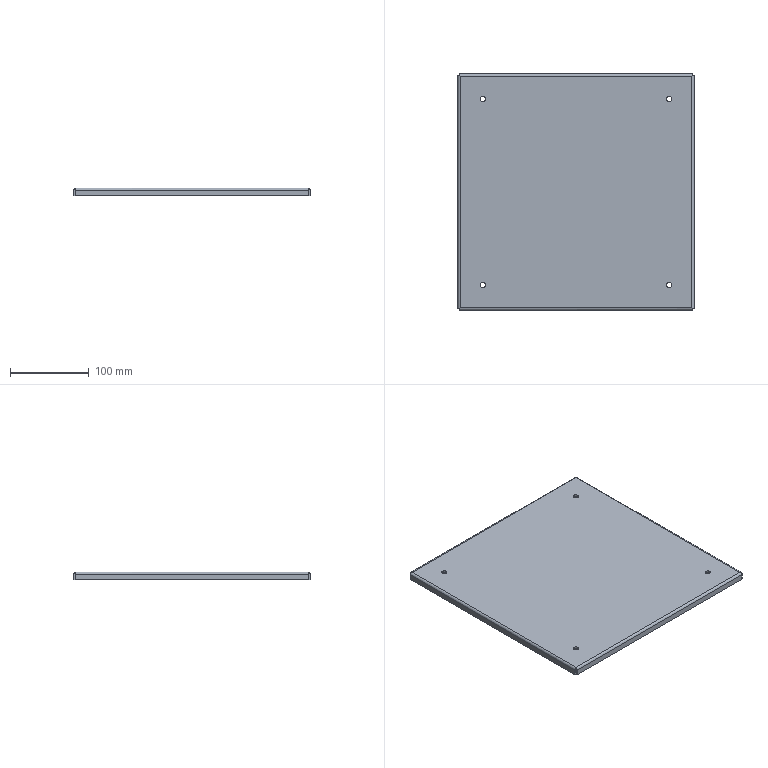Part | STEP file | panel body dalam | 1 solid | 46 faces | box 300 x 300 x 10 mm | volume 177458 mm3 | plane 22 | cylinder 16 | spline 8 | commonest cylinder face diameters 6.6 x8 2 x4 5.6 x4